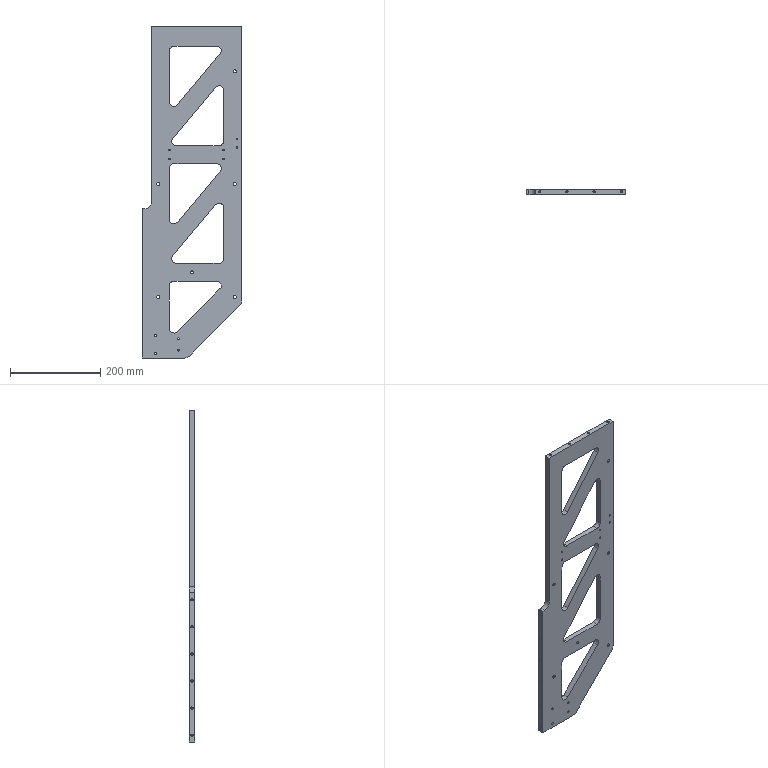Part | SolidWorks | features HoleWzd 8, ICE 2, Chamfer 1, Extrusion 1, Fillet 1 | 1 solid | 116 faces | box 220 x 12 x 735 mm | volume 1211217 mm3 | cylinder 72 | plane 24 | cone 20 | commonest cylinder face diameters 5 x24 20 x17 3.3 x12 6.6 x12 4.2 x4 30 x3